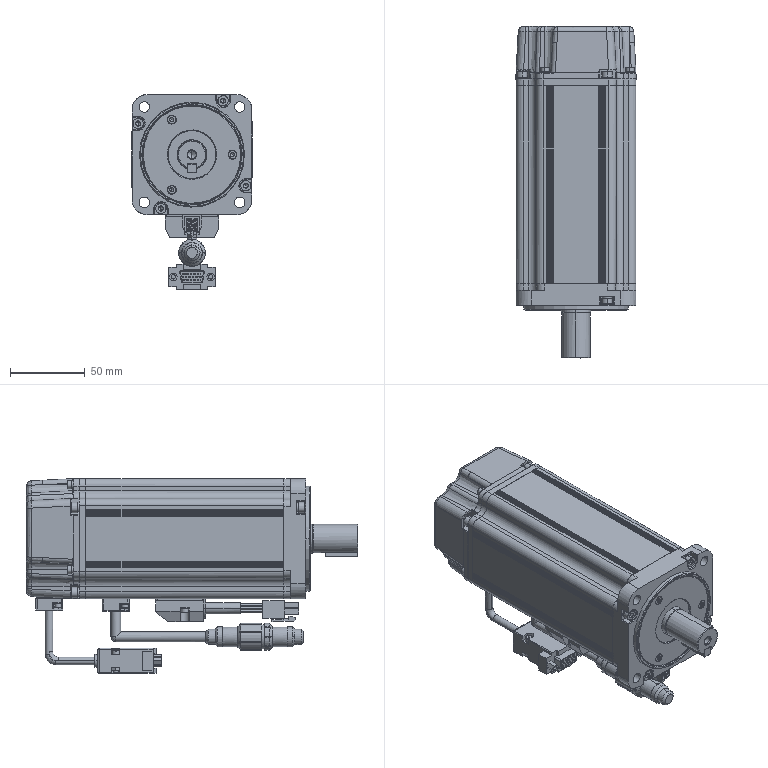Part | NX | features BREP 84 | 59 solids | 3253 faces | volume 406843 mm3 | plane 1486 | cylinder 994 | cone 411 | torus 187 | spline 108 | sphere 67 | commonest cylinder face diameters 2 x142 1 x123 3 x56 2.459 x42 4 x41 7 x40